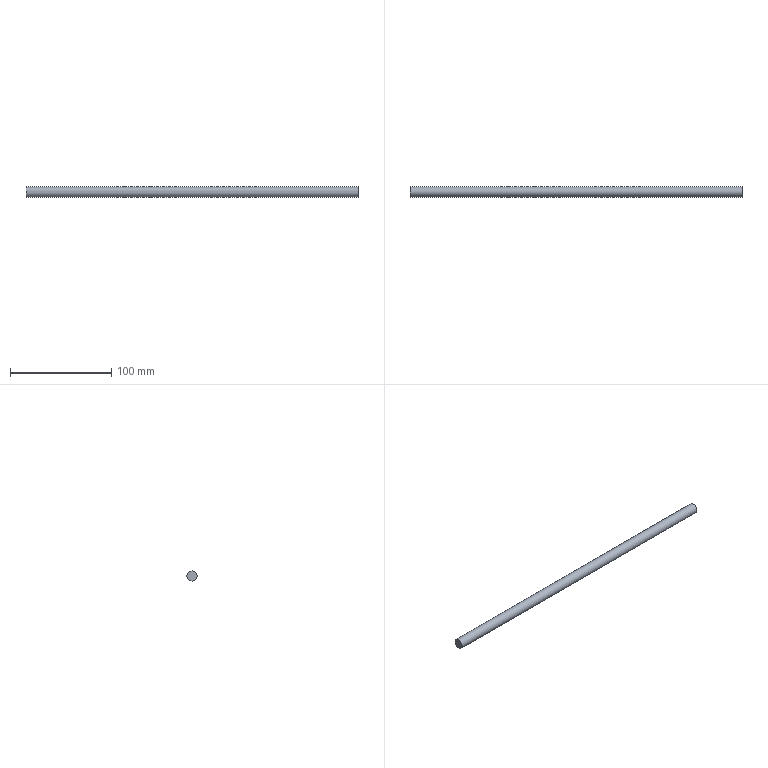Part | NX | features solid 2 | 1 solid | 3 faces | box 328 x 10 x 10 mm | volume 25761 mm3 | plane 2 | cylinder 1 | commonest cylinder face diameters 10 x1
STEP:
#1=CARTESIAN_POINT('',(1175.,436.5,-367.));
#2=VERTEX_POINT('',#1);
#3=CARTESIAN_POINT('',(1175.,436.5,-362.));
#4=DIRECTION('',(1.,0.,0.));
#5=DIRECTION('',(0.,0.,-1.));
#6=AXIS2_PLACEMENT_3D('',#3,#4,#5);
#7=CIRCLE('',#6,5.);
#8=EDGE_CURVE('',#2,#2,#7,.F.);
#9=ORIENTED_EDGE('',*,*,#8,.T.);
#10=EDGE_LOOP('',(#9));
#11=FACE_BOUND('',#10,.T.);
#12=CARTESIAN_POINT('',(1175.,436.5,-362.));
#13=DIRECTION('',(1.,0.,0.));
#14=DIRECTION('',(0.,0.,1.));
#15=AXIS2_PLACEMENT_3D('',#12,#13,#14);
#16=PLANE('',#15);
#17=ADVANCED_FACE('',(#11),#16,.F.);
#18=CARTESIAN_POINT('',(1503.,436.5,-357.));
#19=VERTEX_POINT('',#18);
#20=CARTESIAN_POINT('',(1503.,436.5,-362.));
#21=DIRECTION('',(-1.,0.,0.));
#22=DIRECTION('',(0.,0.,1.));
#23=AXIS2_PLACEMENT_3D('',#20,#21,#22);
#24=CIRCLE('',#23,5.);
#25=EDGE_CURVE('',#19,#19,#24,.F.);
#26=ORIENTED_EDGE('',*,*,#25,.F.);
#27=EDGE_LOOP('',(#26));
#28=FACE_BOUND('',#27,.T.);
#29=ORIENTED_EDGE('',*,*,#8,.F.);
#30=EDGE_LOOP('',(#29));
#31=FACE_BOUND('',#30,.T.);
#32=CARTESIAN_POINT('',(2225.,436.5,-362.));
#33=DIRECTION('',(-1.,0.,0.));
#34=DIRECTION('',(0.,0.,-1.));
#35=AXIS2_PLACEMENT_3D('',#32,#33,#34);
#36=CYLINDRICAL_SURFACE('',#35,5.);
#37=ADVANCED_FACE('',(#28,#31),#36,.T.);
#38=ORIENTED_EDGE('',*,*,#25,.T.);
#39=EDGE_LOOP('',(#38));
#40=FACE_BOUND('',#39,.T.);
#41=CARTESIAN_POINT('',(1503.,431.16,-357.));
#42=DIRECTION('',(-1.,0.,0.));
#43=DIRECTION('',(0.,1.,0.));
#44=AXIS2_PLACEMENT_3D('',#41,#42,#43);
#45=PLANE('',#44);
#46=ADVANCED_FACE('',(#40),#45,.F.);
#47=CLOSED_SHELL('',(#17,#37,#46));
#48=MANIFOLD_SOLID_BREP('',#47);
#49=(LENGTH_UNIT()NAMED_UNIT(*)SI_UNIT(.MILLI.,.METRE.));
#50=UNCERTAINTY_MEASURE_WITH_UNIT(LENGTH_MEASURE(0.00001),#49,'','');
#51=(NAMED_UNIT(*)PLANE_ANGLE_UNIT()SI_UNIT($,.RADIAN.));
#52=(NAMED_UNIT(*)SI_UNIT($,.STERADIAN.)SOLID_ANGLE_UNIT());
#53=(GEOMETRIC_REPRESENTATION_CONTEXT(3)GLOBAL_UNCERTAINTY_ASSIGNED_CONTEXT((#50))GLOBAL_UNIT_ASSIGNED_CONTEXT((#49,#51,#52))REPRESENTATION_CONTEXT('',''));
#54=ADVANCED_BREP_SHAPE_REPRESENTATION('',(#48),#53);